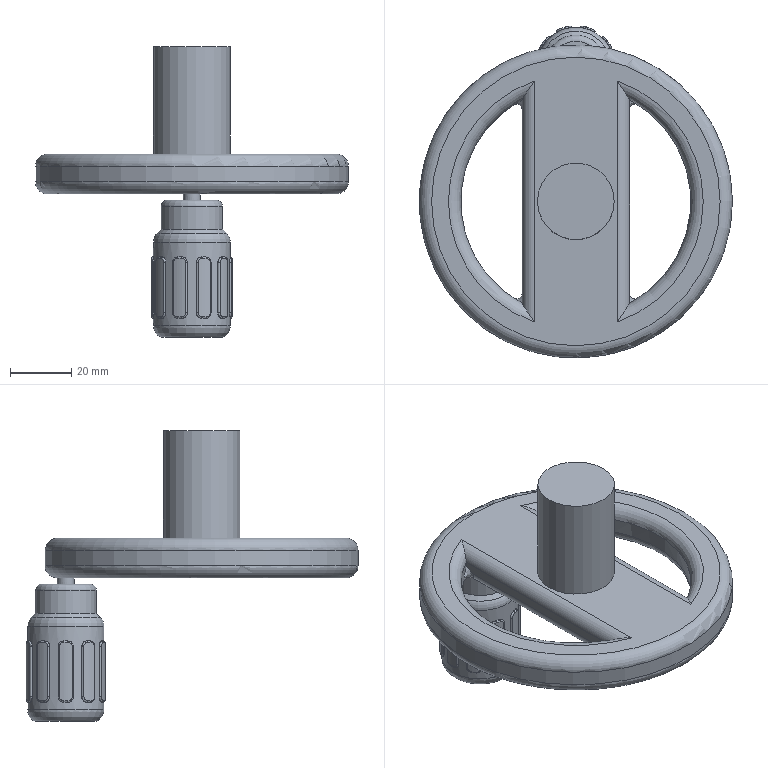Part | STEP file | DEWALT-DWE7294-B3-01 | 1 solid | 276 faces | box 102 x 108.2 x 94.708 mm | volume 107862 mm3 | spline 84 | cylinder 75 | plane 65 | torus 39 | sphere 12 | cone 1 | commonest cylinder face diameters 1 x38 2 x12 26.2 x10 8 x5 20 x2 25 x2